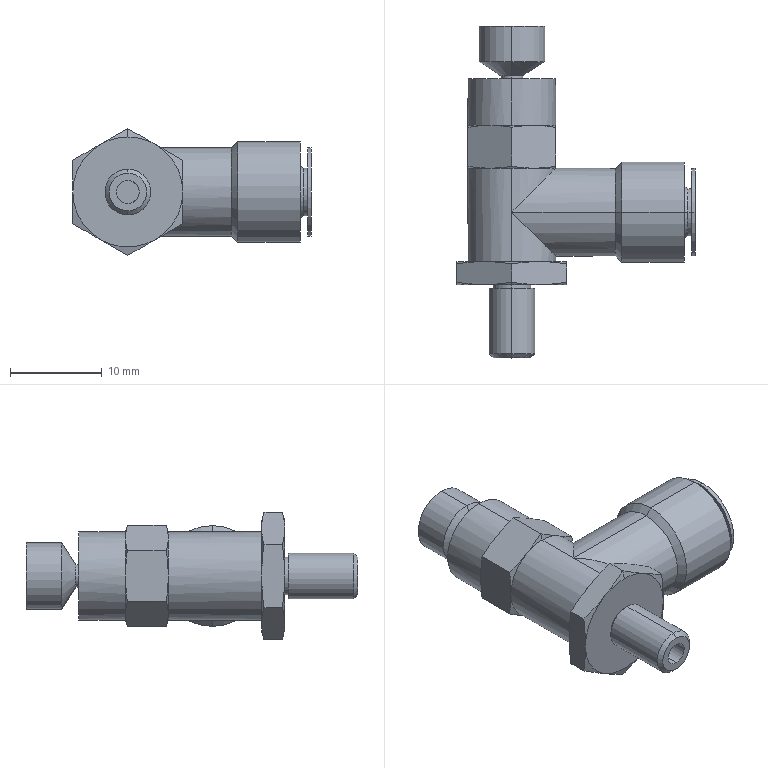Part | STEP file | SPCN4_M5_B_SPCN4-M5-B | 1 solid | 88 faces | box 26 x 36.2 x 13.856 mm | volume 3077 mm3 | cone 36 | cylinder 28 | plane 24 | commonest cylinder face diameters 9.6 x10 2.48 x4 2.4 x2 4 x2 4.134 x2 5 x2